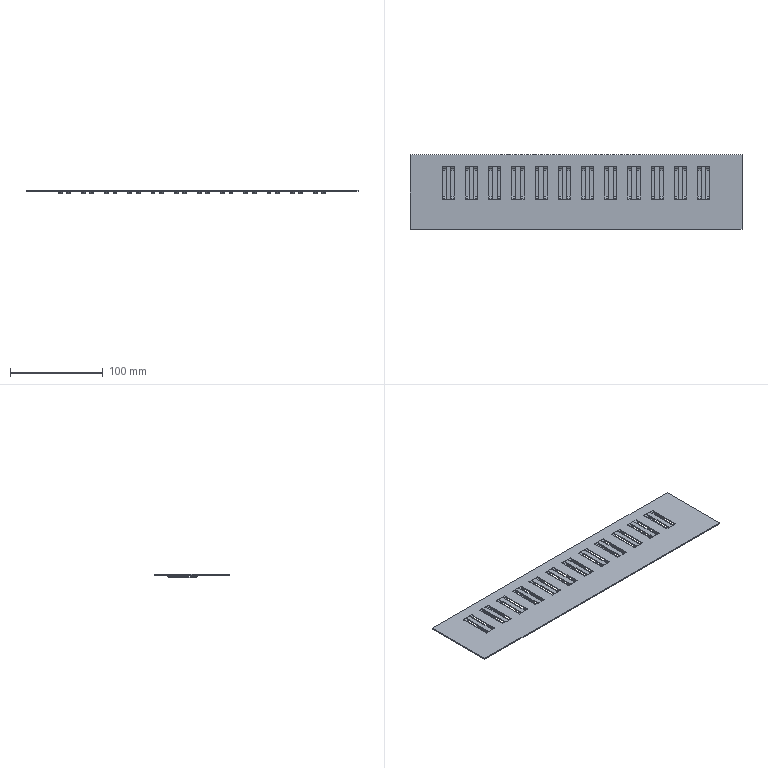Part | SolidWorks | features FlatPattern 1, FormToolInstance 1, LPattern 1, SMBaseFlange 1, SheetMetal 1 | 1 solid | 510 faces | box 357.6 x 80 x 4.201 mm | volume 34630 mm3 | plane 318 | cylinder 192 | commonest cylinder face diameters 4 x96 1.6 x48 6.4 x48